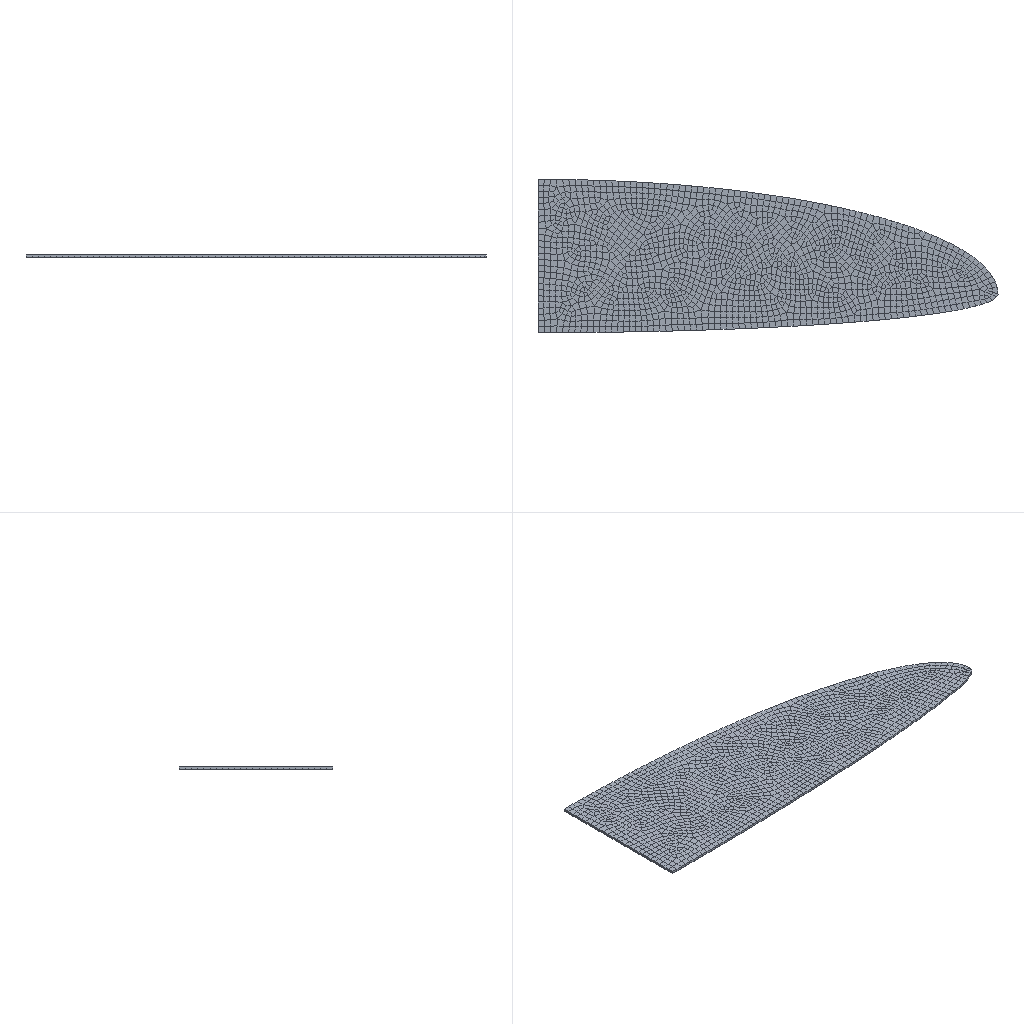Simulation study | abaqus
Set-up summary:
category,name,step,type,value,unit,region
solver,abaqus,,Abaqus/CAE 2024
units,SI m-kg-s (Pa),,inferred,E=7e+10 density=2700
analysis,Step-1,,dynamic explicit,nlgeom=True; time_period=1
mesh,nodes,,,3917
mesh,elements,,,1866
element_type,C3D8R,,,1866
material,Material-1,,E,7e+10
material,Material-1,,nu,0.3
material,Material-1,,density,2700
section,Material-1,,solid section,,,_PickedSet12
bc,BC-1,Step-1,fixed,"[dofs=rx,rz,x,y,z n=5]",,_PickedSet34
bc,BC-1,Step-1,displacement,1 [dofs=ry],,_PickedSet34
constraint,coupling,,,1
Abaqus input file, long lists of numbers shortened:
*Heading
** Job name: deck Model name: Model-1-Copy-Copy
** Generated by: Abaqus/CAE 2024
*Preprint, echo=NO, model=NO, history=NO, contact=NO
**
** PARTS
**
*Part, name=wing
*End Part
**
**
** ASSEMBLY
**
*Assembly, name=Assembly
**
*Instance, name=wing-1, part=wing
*Node
      1, 0.07456, 0.002034, 0.0004
      2, 0.0735, 0.003736, 0.0004
** (3914 more lines like these left out)
*Element, type=C3D8R
   1, 1608, 1617,  138, 1609, 3566, 3575, 2096, 3567
   2,    1, 1610,  578,  420, 1959, 3568, 2536, 2378
** (1864 more lines like these left out)
*Node
   3917,           0., 0.00625,           0.
*Nset, nset=wing-1-RefPt_, internal
3917,
*Nset, nset=_PickedSet12, internal, generate
    1,  3916,     1
*Elset, elset=_PickedSet12, internal, generate
    1,  1866,     1
** Section: Section-1
*Solid Section, elset=_PickedSet12, controls=EC-1, material=Material-1
,
*End Instance
**
*Nset, nset=b_Set-3, instance=wing-1, generate
    1,  3916,     1
*Elset, elset=b_Set-3, instance=wing-1, generate
    1,  1866,     1
*Nset, nset=_PickedSet32, internal, instance=wing-1
 3917,
*Nset, nset=_PickedSet34, internal, instance=wing-1
 3917,
*Elset, elset=__PickedSurf33_S4, internal, instance=wing-1
  36,  38,  39, 184, 185, 207, 208, 209, 210, 211, 212, 457, 536, 674, 675, 676
*Elset, elset=__PickedSurf33_S6, internal, instance=wing-1
  37, 181, 182, 200, 201, 206, 673, 677
*Elset, elset=__PickedSurf33_S5, internal, instance=wing-1
 183,
*Surface, type=ELEMENT, name=_PickedSurf33, internal
__PickedSurf33_S4, S4
__PickedSurf33_S6, S6
__PickedSurf33_S5, S5
** Constraint: Constraint-1
*Coupling, constraint name=Constraint-1, ref node=_PickedSet32, surface=_PickedSurf33
*Kinematic
*End Assembly
**
** ELEMENT CONTROLS
**
*Section Controls, name=EC-1, DISTORTION CONTROL=YES, length ratio=0.5, hourglass=STIFFNESS
1., 1., 1.
*Amplitude, name=Amp-1, time=TOTAL TIME, definition=PERIODIC
1,           18.84,              0.,              0.
             0., 0.3663
**
** MATERIALS
**
*Material, name=Material-1
*Density
2700.,
*Elastic
 7e+10, 0.3
** ----------------------------------------------------------------
**
** STEP: Step-1
**
*Step, name=Step-1, nlgeom=YES
*Dynamic, Explicit
, 1.
*Bulk Viscosity
0.06, 1.2
** Mass Scaling: Semi-Automatic
**               Whole Model
*Fixed Mass Scaling, factor=1000.
**
** BOUNDARY CONDITIONS
**
** Name: BC-1 Type: Displacement/Rotation
*Boundary, amplitude=Amp-1
_PickedSet34, 1, 1
_PickedSet34, 2, 2
_PickedSet34, 3, 3
_PickedSet34, 4, 4
_PickedSet34, 5, 5, 1.
_PickedSet34, 6, 6
**
** OUTPUT REQUESTS
**
*Restart, write, number interval=1, time marks=NO
**
** FIELD OUTPUT: F-Output-1
**
*Output, field, variable=PRESELECT
**
** HISTORY OUTPUT: H-Output-1
**
*Output, history, variable=PRESELECT
*End Step
Results summary:
result,odb.job_status,,,JOB_STATUS_UNKNOWN,"consistent, unstated (Abaqus has no unit system)"
result,steps[0].procedure,Step-1,,"*DYNAMIC, EXPLICIT","consistent, unstated (Abaqus has no unit system)"
result,steps[0].time_period,Step-1,,1,"consistent, unstated (Abaqus has no unit system)"
result,steps[0].n_frames,Step-1,,16,"consistent, unstated (Abaqus has no unit system)"
result,steps[0].last_frame.id,Step-1,,514452,"consistent, unstated (Abaqus has no unit system)"
result,steps[0].last_frame.value,Step-1,,0.75,"consistent, unstated (Abaqus has no unit system)"
result,steps[0].last_frame.description,Step-1,,Increment    514452: Step Time =   0.75,"consistent, unstated (Abaqus has no unit system)"
result,steps[0].completed,Step-1,,False,"consistent, unstated (Abaqus has no unit system)"
result,steps[0].max_U_magnitude,Step-1,,0.02876,"consistent, unstated (Abaqus has no unit system)"
result,steps[0].max_S_mises,Step-1,,1.4347e+09,"consistent, unstated (Abaqus has no unit system)"
result,steps[0].RF_sum[1],Step-1,,48.244,"consistent, unstated (Abaqus has no unit system)"
result,steps[0].RF_sum[2],Step-1,,-27.528,"consistent, unstated (Abaqus has no unit system)"
result,steps[0].RF_sum[3],Step-1,,-43.177,"consistent, unstated (Abaqus has no unit system)"
result,steps[0].diagnostic.n_increments,Step-1,,20,"consistent, unstated (Abaqus has no unit system)"